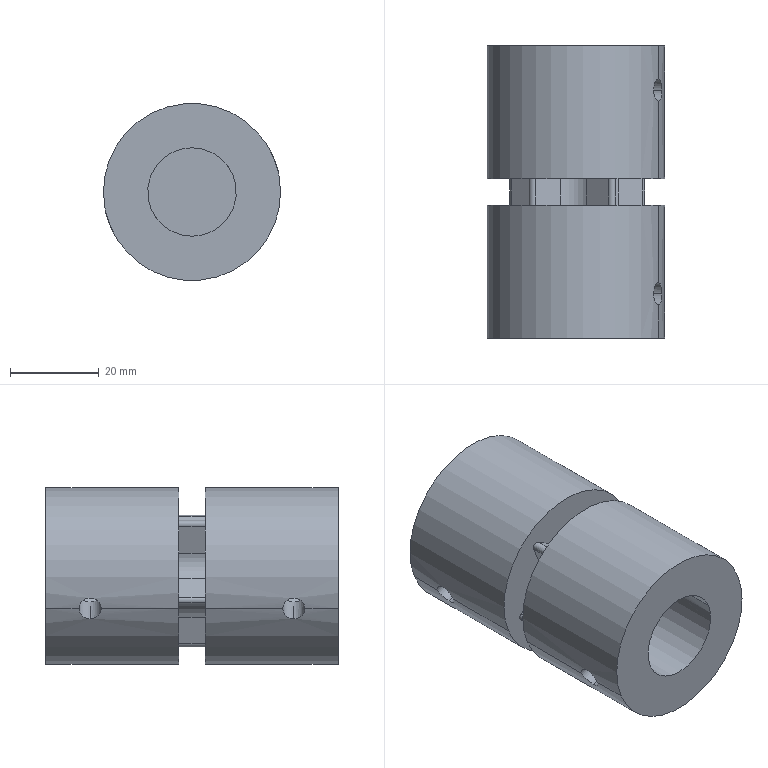Part | STEP file | Cut-Extrude 7 | 1 solid | 46 faces | box 40 x 66 x 40 mm | volume 67445 mm3 | cylinder 30 | plane 16 | commonest cylinder face diameters 2 x8 5 x8 10 x6 20 x4 40 x4